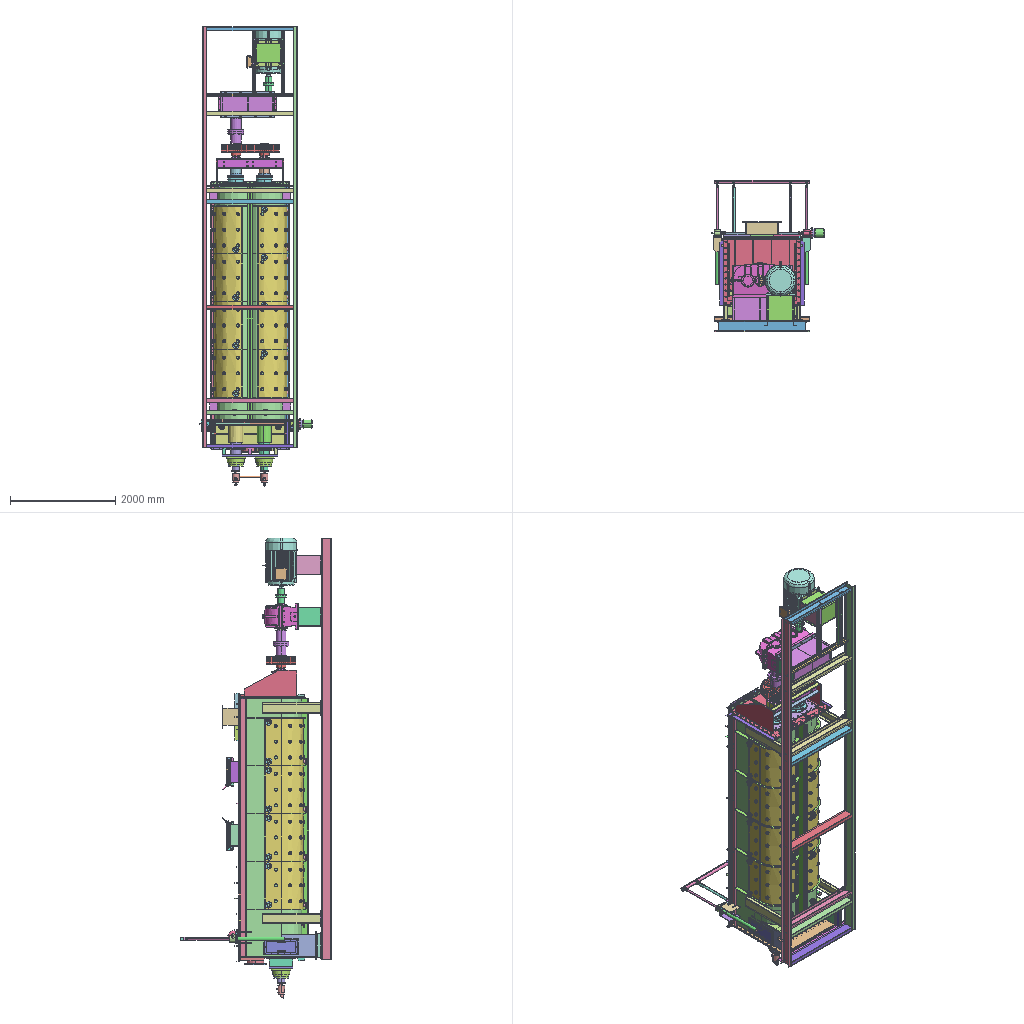Assembly | SolidWorks | 78 different items | 255 placed | box 2141 x 2886 x 8740 mm
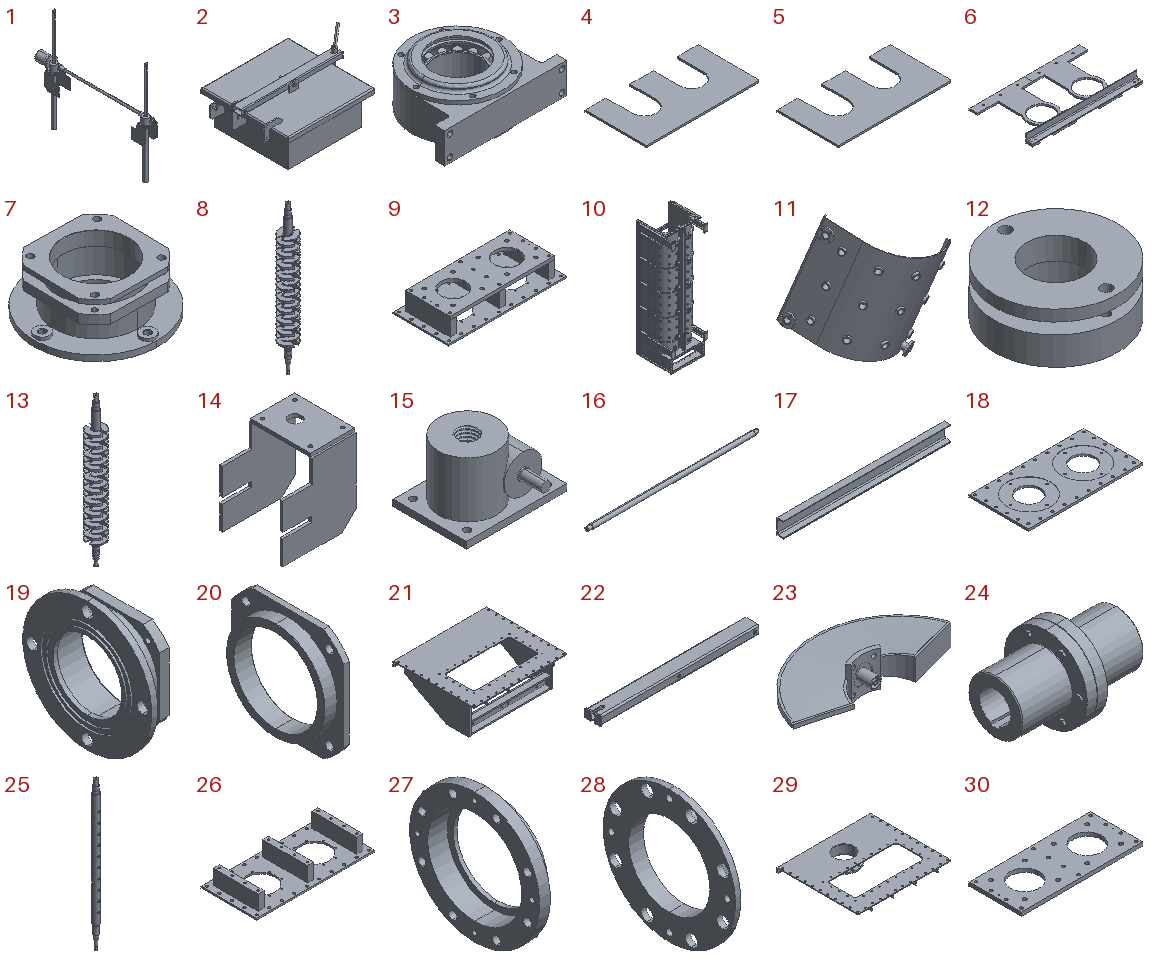Parts list (item | name | quantity | parent item | size | volume | features):
1 | (subassembly) | x1 | - | 241 x 2141 x 1901 mm | 19247413 mm3 | features AEMSimFeature 1
2 | (subassembly) | x2 | - | 610.405 x 476 x 304.855 mm | 2318365 mm3 | features AEMSimFeature 1, CompositeCurve 1
3 | (subassembly) | x2 | - | 480 x 370 x 194.8 mm | 12671030 mm3 | -
4 | (subassembly) | x1 | - | 1290 x 700 x 80 mm | 13949366 mm3 | features AEMSimFeature 1
5 | (subassembly) | x1 | in 4 | 1290 x 700 x 80 mm | 13949366 mm3 | features AEMSimFeature 1, MirrorCompFeat 1, ReferencePattern 1
6 | (subassembly) | x1 | - | 1300 x 750 x 100 mm | 9468918 mm3 | features HoleWzd 2, LPattern 2, AEMSimFeature 1
7 | (subassembly) | x2 | - | 420 x 420 x 162 mm | 4466169 mm3 | features ReferencePattern 3, AEMSimFeature 1, LocalCirPattern 1
8 | (subassembly) | x1 | - | - | 287612540 mm3 | features ReferencePattern 36, LocalLPattern 4, AEMSimFeature 1, RefAxis 1
9 | (subassembly) | x1 | - | 1185 x 560 x 198 mm | 31946209 mm3 | features AEMSimFeature 1
10 | (subassembly) | x1 | - | 1600 x 1565 x 4990 mm | 308843646 mm3 | features ReferencePattern 19, LocalLPattern 6, MirrorCompFeat 3, AEMSimFeature 1
11 | (subassembly) | x8 | in 10 | 940.727 x 808.112 x 1146 mm | 7168589 mm3 | features ReferencePattern 10, LocalLPattern 2, AEMSimFeature 1, LocalCirPattern 1, MirrorCompFeat 1
12 | (subassembly) | x2 | - | 110 x 110 x 45 mm | 226861 mm3 | features AEMSimFeature 1
13 | (subassembly) | x1 | - | - | 286429521 mm3 | features ReferencePattern 36, LocalLPattern 4, CompositeCurve 2, AEMSimFeature 1, RefAxis 1
14 | - | x1 | in 1 | 258 x 222 x 292 mm | 1584806 mm3 | features ICE 2, Chamfer 1, Cut 1, Extrusion 1, HoleWzd 1, MirrorSolid 1
15 | - | x1 | in 1 | - | 2041758 mm3 | features ICE 6, Extrusion 1, Helix 1, MirrorSolid 1, RefAxis 1, SweepCut 1
16 | - | x1 | in 1 | 1476 x 40 x 40 mm | 1810594 mm3 | features Chamfer 1, ICE 1, MirrorPattern 1, Revolution 1
17 | - | x3 | in 10 | 1300 x 53 x 120 mm | 1996260 mm3 | features WeldMemberFeat 1, WeldmentFeature 1
18 | - | x1 | - | 1140 x 590 x 22 mm | 12045594 mm3 | features ICE 3, CirPattern 2, HoleWzd 2, RefAxis 2, Extrusion 1
19 | - | x2 | in 7 | 116 x 420 x 420 mm | 3215271 mm3 | features ICE 4, Chamfer 2, CirPattern 2, HoleWzd 1, RefAxis 1, Revolution 1
20 | - | x2 | in 7 | 48 x 300 x 300 mm | 1152473 mm3 | features Chamfer 3, ICE 2, CirPattern 1, RefAxis 1, Revolution 1
21 | - | x1 | - | 1448 x 1250 x 512 mm | 47295525 mm3 | features ICE 13, LPattern 8, Chamfer 5, HoleWzd 4, MirrorPattern 3, MirrorSolid 2, Extrusion 1, Fillet 1
22 | - | x2 | in 2 | 554 x 54 x 30.061 mm | 237150 mm3 | features Cut 2, ICE 2, MirrorSolid 1, WeldMemberFeat 1, WeldmentFeature 1
23 | - | x80 | in 8, 13 | 715.716 x 337.387 x 160 mm | 3757176 mm3 | features ICE 17, MoveFace 13, DeleteBody 4, Chamfer 2, OffsetRefSurface 2, Split 2, Thicken 2, Blend 1, CirPattern 1, CombineBodies 1, Extrusion 1, MirrorSolid 1, Punch 1, RefAxis 1, RevCut 1, WeldmentFeature 1
24 | - | x1 | - | 294 x 200 x 200 mm | 3610457 mm3 | features ICE 15, Chamfer 6, Revolution 3, CirPattern 2, Fillet 2
25 | - | x1 | in 8 | 265 x 265 x 6370 mm | 136126152 mm3 | features ICE 15, LPattern 6, MirrorPattern 5, Fillet 2, HoleWzd 2, MoveFace 2, RefAxis 2, Chamfer 1, CombineBodies 1, Extrusion 1, MoveCopyBody 1, Revolution 1, Split 1, WeldBeadFeat 1, WeldmentFeature 1
26 | - | x1 | in 9 | 1185 x 560 x 166 mm | 20349216 mm3 | features ICE 3, HoleWzd 2, LPattern 2, CirPattern 1, Extrusion 1, MirrorPattern 1, RefAxis 1
27 | - | x2 | - | 65 x 365 x 365 mm | 1770977 mm3 | features CirPattern 1, HoleWzd 1, ICE 1, RefAxis 1, Revolution 1
28 | - | x3 | - | 41 x 365 x 365 mm | 1248338 mm3 | features ICE 2, Revolution 1
29 | - | x1 | - | 1448 x 1250 x 147 mm | 19462200 mm3 | features ICE 12, LPattern 7, Chamfer 4, MirrorPattern 2, MirrorSolid 2, Extrusion 1, Fillet 1, HoleWzd 1
30 | - | x1 | in 9 | 1050 x 450 x 32 mm | 11596993 mm3 | features ICE 3, MirrorPattern 3, CirPattern 1, Extrusion 1, HoleWzd 1
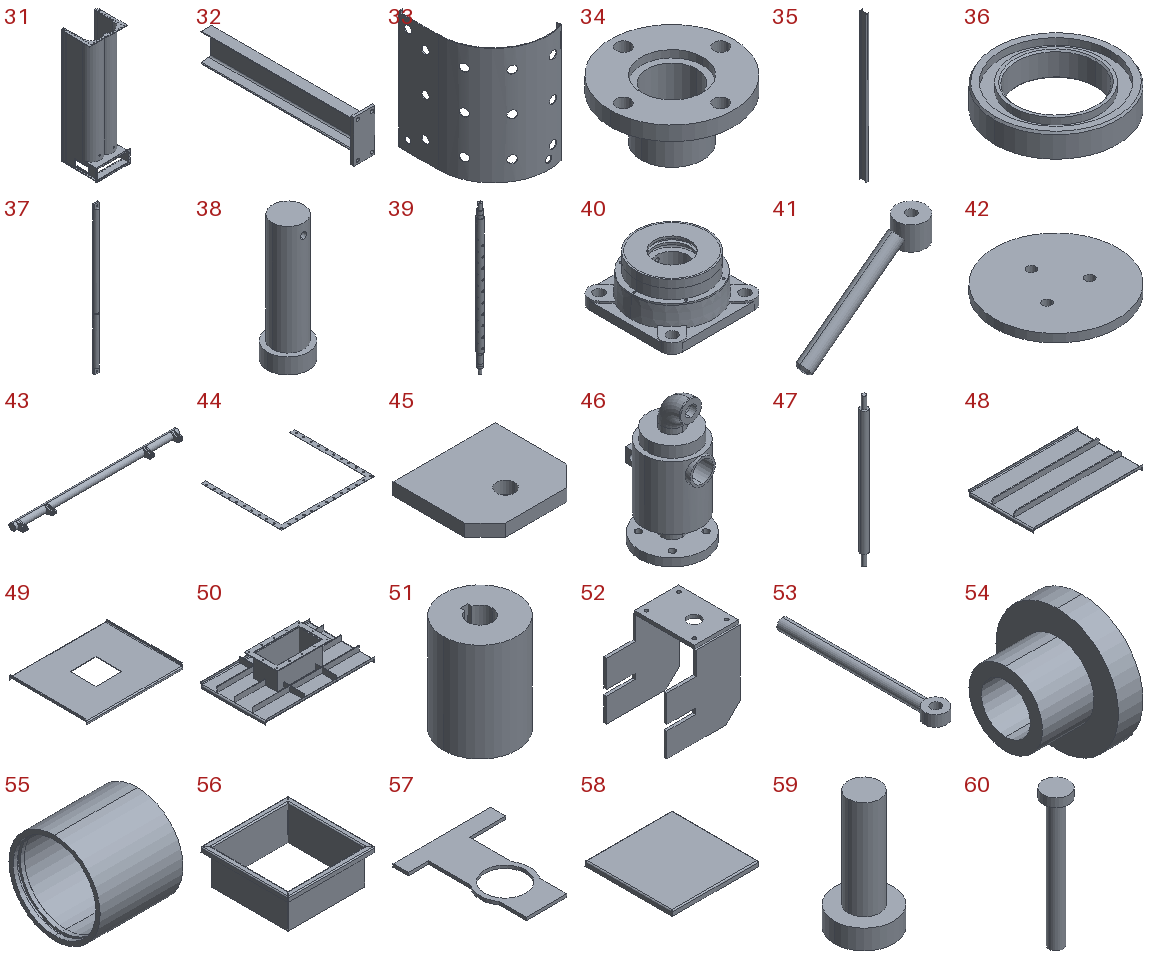31 | - | x1 | in 10 | 1600 x 1465 x 4987 mm | 200673004 mm3 | features ICE 14, HoleWzd 6, MirrorPattern 6, LPattern 5, CombineBodies 3, MirrorSolid 3, MoveFace 3, Extrusion 1, MoveCopyBody 1, Split 1
32 | - | x4 | in 10 | 150 x 1120 x 300 mm | 4040615 mm3 | features HoleWzd 1, ICE 1, MirrorPattern 1, WeldMemberFeat 1, WeldmentFeature 1
33 | - | x8 | in 11 | 548.116 x 742 x 900 mm | 6001500 mm3 | features EdgeFlange 2, ICE 2, RevCut 2, CirPattern 1, FlatPattern 1, LPattern 1, SMBaseFlange 1, SheetMetal 1
34 | - | x26 | in 10, 11 | 120 x 120 x 57 mm | 161025 mm3 | features ExtruThin 1, HoleWzd 1, ICE 1
35 | - | x1 | in 10 | 100 x 200 x 4480 mm | 12833917 mm3 | features Extrusion 1, MoveFace 1
36 | - | x3 | in 8, 13 | 85 x 85 x 17 mm | 42385 mm3 | features Chamfer 2, ICE 2, Extrusion 1
37 | - | x2 | - | 50 x 50 x 1600 mm | 3004412 mm3 | features HoleWzd 2, ICE 2, MirrorPattern 2, Extrusion 1
38 | - | x2 | - | 26 x 26 x 80 mm | 27050 mm3 | features ICE 2, Extrusion 1
39 | - | x1 | in 13 | 265 x 265 x 6190 mm | 134783572 mm3 | features ICE 16, HoleWzd 4, LPattern 4, MirrorPattern 4, Chamfer 2, CombineBodies 2, Fillet 2, MoveFace 2, RefAxis 2, CirPattern 1, DeleteBody 1, Extrusion 1, MoveCopyBody 1, Revolution 1, Split 1, WeldmentFeature 1
40 | - | x2 | - | 370 x 370 x 185 mm | 8271965 mm3 | features Revolution 5, RevCut 3, Boss 2, CirPattern 2, ICE 2, Cut 1, Extrusion 1, HoleWzd 1, RevolutionThin 1
41 | - | x2 | in 2 | 107.206 x 25 x 73.855 mm | 19838 mm3 | features Chamfer 1, Extrusion 1, HoleWzd 1, Revolution 1
42 | - | x1 | in 13 | 150 x 150 x 10 mm | 173864 mm3 | features BaseBody 1
43 | - | x1 | - | 1806 x 139 x 73 mm | 3217271 mm3 | features ICE 3, LPattern 2, MirrorSolid 2, HoleWzd 1, WeldMemberFeat 1, WeldmentFeature 1
44 | - | x2 | in 10 | 1448 x 1250 x 3 mm | 798363 mm3 | features Extrusion 1
45 | - | x2 | in 2 | 50 x 45 x 6 mm | 12518 mm3 | features Chamfer 1, Cut 1, Extrusion 1
46 | - | x2 | - | 150 x 170 x 315 mm | 2389466 mm3 | features ICE 8, CirPattern 1, Extrusion 1, HoleWzd 1, Sweep 1, SweepCut 1
47 | - | x1 | - | 30 x 30 x 615 mm | 384138 mm3 | features ICE 2, Extrusion 1
48 | - | x2 | - | 1492 x 898 x 110 mm | 11274482 mm3 | features Chamfer 2, EdgeFlange 2, BossThin 1, FlatPattern 1, SMBaseFlange 1, SheetMetal 1, WeldmentFeature 1
49 | - | x2 | - | 1492 x 1200 x 74 mm | 10683181 mm3 | features EdgeFlange 2, FlatPattern 1, ICE 1, SMBaseFlange 1, SheetMetal 1
50 | - | x1 | - | 1492 x 898 x 350 mm | 16578129 mm3 | features BossThin 2, EdgeFlange 2, HoleWzd 2, MirrorSolid 2, Cut 1, FlatPattern 1, ICE 1, LPattern 1, MirrorPattern 1, SMBaseFlange 1, SheetMetal 1
51 | - | x2 | in 1 | 60 x 60 x 80 mm | 183532 mm3 | features ICE 4, Extrusion 1
52 | - | x1 | in 1 | 258 x 222 x 292 mm | 1584806 mm3 | features ICE 2, Chamfer 1, Cut 1, Extrusion 1, HoleWzd 1, MirrorSolid 1
53 | - | x2 | in 2 | 20 x 150 x 10 mm | 12716 mm3 | features Extrusion 1, ICE 1, Revolution 1
54 | - | x8 | in 7 | 31 x 50 x 50 mm | 24606 mm3 | features Chamfer 1, Revolution 1
55 | - | x2 | in 8, 13 | 200 x 220 x 220 mm | 1255193 mm3 | features ICE 2, Revolution 1
56 | - | x2 | in 2 | 460 x 460 x 183 mm | 1117648 mm3 | features FlatPattern 4, ICE 1, SMBaseFlange 1, SMMiteredFlange 1, SheetMetal 1
57 | - | x2 | in 6 | 650 x 750 x 20 mm | 3819673 mm3 | features ICE 2, Extrusion 1
58 | - | x2 | in 2 | 476 x 476 x 28 mm | 807964 mm3 | features CornerFeat 4, FlatPattern 1, SMBaseFlange 1, SMMiteredFlange 1, SheetMetal 1
59 | - | x4 | in 2 | 15 x 15 x 30 mm | 2140 mm3 | features Extrusion 1, ICE 1
60 | - | x4 | in 2 | 15 x 15 x 80 mm | 4653 mm3 | features Extrusion 1, ICE 1
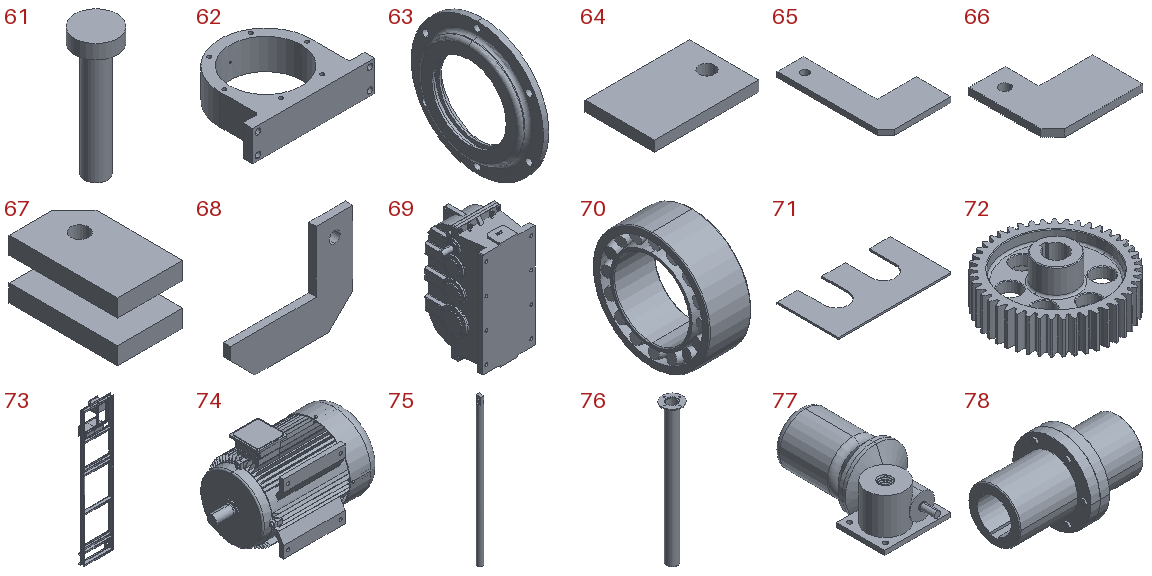61 | - | x2 | in 2 | 15 x 15 x 45 mm | 2894 mm3 | features Extrusion 1, ICE 1
62 | - | x2 | in 3 | 480 x 370 x 120 mm | 7370776 mm3 | features HoleWzd 3, ICE 2, CirPattern 1, Extrusion 1, Fillet 1, RefAxis 1
63 | - | x4 | in 3 | 47.4 x 360 x 360 mm | 1531898 mm3 | features ICE 1, Revolution 1
64 | - | x2 | in 2 | 60 x 40 x 6 mm | 14018 mm3 | features Extrusion 1, ICE 1
65 | - | x2 | in 2 | 75 x 125 x 6 mm | 32618 mm3 | features Chamfer 1, Extrusion 1, ICE 1
66 | - | x2 | in 2 | 75 x 70 x 6 mm | 23195 mm3 | features Chamfer 1, Extrusion 1, ICE 1
67 | - | x2 | in 5 | 60 x 100 x 54 mm | 178758 mm3 | features Chamfer 1, Extrusion 1, ICE 1, MirrorSolid 1
68 | - | x2 | in 2 | 100 x 6 x 80 mm | 24218 mm3 | features Chamfer 2, Extrusion 1, ICE 1
69 | - | x1 | - | 780 x 662 x 1105 mm | 238167448 mm3 | features ICE 43, Extrusion 14, Fillet 9, CirPattern 5, Chamfer 4, MirrorPattern 4, DeleteBody 2, LPattern 1, RefAxis 1, Revolution 1
70 | - | x2 | in 3 | 100 x 280 x 280 mm | 2236455 mm3 | features Revolution 4, Fillet 2, CirPattern 1, MirrorPattern 1, MirrorSolid 1
71 | - | x1 | in 5 | 1290 x 700 x 20 mm | 13591851 mm3 | features Extrusion 1, Fillet 1, ICE 1
72 | - | x2 | - | 563.903 x 563.597 x 220 mm | 18785882 mm3 | features ICE 8, Chamfer 2, CirPattern 1, Extrusion 1, Fillet 1, RefAxis 1
73 | - | x1 | - | 1791 x 685 x 8000 mm | 140497975 mm3 | features MoveFace 19, MoveCopyBody 18, ICE 10, MirrorSolid 9, WeldMemberFeat 7, 3DProfileFeature 3, Cut 3, DeleteBody 2, Shell 2, Punch 1, WeldmentFeature 1
74 | - | x1 | - | 1055 x 665 x 715 mm | 197436858 mm3 | features Boss 17, Cut 5, Revolution 5, Fillet 4, Chamfer 3, CirPattern 3, RevCut 2, 3DProfileFeature 1, LPattern 1, MirrorPattern 1, MoveCopyBody 1
75 | - | x2 | in 1 | 40 x 40 x 1100 mm | 1353457 mm3 | features ICE 2, Extrusion 1
76 | - | x2 | in 1 | 130 x 130 x 909 mm | 633307 mm3 | features ICE 2, ExtruThin 1, HoleWzd 1
77 | - | x1 | in 1 | 236 x 443.1 x 200 mm | 7884853 mm3 | features ICE 9, Blend 2, Fillet 2, Extrusion 1, Helix 1, RefAxis 1, SweepCut 1
78 | - | x1 | - | 474 x 300 x 300 mm | 12928515 mm3 | features ICE 15, Chamfer 6, Revolution 3, CirPattern 2, Fillet 2
Mates (type | each side: item.copy, entity, surface, feature):
In the top assembly
Coincident | 44.1 face plane Boss-Extrude1 | 21.1 face plane Boss-Extrude1
Concentric | 31.1 face cylinder M22 Tapped Hole3 | 21.1 face cylinder Cut-Extrude2
Concentric | 31.1 face cylinder Mirror4 | 21.1 face cylinder Cut-Extrude2
Coincident | 44.2 face plane Boss-Extrude1 | 29.1 face plane Boss-Extrude1
Concentric | 31.1 face cylinder M22 Tapped Hole1 | 29.1 face cylinder Cut-Extrude2
Concentric | 31.1 face cylinder LPattern1 | 29.1 face cylinder Cut-Extrude2
Coincident | 27.1 face plane Revolve1 | 28.1 face plane Revolve1
Concentric | 27.1 face cylinder Revolve1 | 28.1 face cylinder Revolve1
DistanceDim | 27.2 face plane Revolve1 | 28.2 face plane Revolve1
Concentric | 27.2 face cylinder Revolve1 | 28.2 face cylinder Revolve1
DistanceDim | assembly face | assembly face
Concentric | assembly face | assembly face
DistanceDim | 28.3 face plane Revolve1 | 27.1 face plane Revolve1
Concentric | 27.1 face cylinder Revolve1 | 28.3 face cylinder Revolve1
DistanceDim | 25.1 face plane Boss-Extrude7 | 18.1 face plane Boss-Extrude1
DistanceDim | 39.1 face plane Boss-Extrude7 | 18.1 face plane Boss-Extrude1
Concentric | 39.1 face cylinder Boss-Extrude4 | 70.1 face cylinder Revolve1
Coincident | 39.1 face plane Boss-Extrude5 | 70.1 face plane Revolve1
Concentric | 25.1 face cylinder Boss-Extrude1 | 70.2 face cylinder Revolve1
Coincident | 25.1 face plane Boss-Extrude5 | 70.2 face plane Revolve1
DistanceDim | 26.1 face plane Boss-Extrude1 | 29.1 face plane Boss-Extrude1
Concentric | 29.1 face cylinder M20 Tapped Hole1 | 26.1 face cylinder Cut-Extrude1
Concentric | 29.1 face cylinder LPattern12 | 26.1 face cylinder Cut-Extrude1
DistanceDim | 27.2 face plane Revolve1 | 26.1 face plane Boss-Extrude1
Concentric | 26.1 face cylinder Cut-Extrude2 | 27.2 face cylinder Revolve1
Concentric | 26.1 face cylinder Mirror1 | 27.2 face cylinder Cut-Extrude1
DistanceDim | 27.1 face plane Revolve1 | 26.1 face plane Boss-Extrude1
Concentric | 26.1 face cylinder Cut-Extrude2 | 27.1 face cylinder Revolve1
Concentric | 30.1 face cylinder Mirror3 | 40.1 face cylinder Base-Extrude
Concentric | 30.1 face cylinder Mirror1 | 40.1 face cylinder Base-Extrude
Coincident | 30.1 face plane Boss-Extrude1 | 40.1 face plane Base-Extrude
Concentric | 30.1 face cylinder M36 Tapped Hole1 | 40.2 face cylinder Base-Extrude
Concentric | 30.1 face cylinder CirPattern1 | 40.2 face cylinder Base-Extrude
Coincident | 30.1 face plane Boss-Extrude1 | 40.2 face plane Base-Extrude
Concentric | 25.1 face cylinder Revolve2 | 46.1 face cylinder Cut-Extrude2
Parallel | 30.1 face plane Boss-Extrude1 | 46.1 face plane Boss-Extrude4
Coincident | 25.1 face plane Revolve2 | 46.1 face plane Boss-Extrude1
Concentric | 39.1 face cylinder Revolve1 | 46.2 face cylinder Sweep1
Parallel | 30.1 face plane Boss-Extrude1 | 46.2 face plane Boss-Extrude4
Coincident | 39.1 face plane Revolve1 | 46.2 face plane Boss-Extrude1
Concentric | 46.2 face cylinder Cut-Extrude5 | 47.1 face cylinder Boss-Extrude1
Coincident | 46.2 face plane Boss-Extrude4 | 47.1 face plane Boss-Extrude1
Parallel | 31.1 face plane Boss-Extrude6 | 57.1 face plane
Coincident | 31.1 face plane Boss-Extrude3 | 57.1 face plane
DistanceDim | 31.1 face plane Mirror2 | 48.1 face plane Base-Flange1
Coincident | 17.1 edge | 48.1 face plane Edge-Flange2
Width | 48.1 face plane Edge-Flange3 | 48.1 face plane Edge-Flange3 | 31.1 face plane Boss-Extrude1 | 31.1 face plane Boss-Extrude1
Coincident | 48.1 face plane Edge-Flange3 | 49.1 face plane Edge-Flange3
Coincident | 48.1 face plane Edge-Flange2 | 49.1 face plane Edge-Flange2
Coincident | 48.1 face plane Base-Flange1 | 49.1 face plane Base-Flange1
Coincident | 49.2 face plane Base-Flange1 | 50.1 face plane Base-Flange1
Coincident | 49.2 face plane Edge-Flange3 | 50.1 face plane Edge-Flange3
Coincident | 49.2 face plane Edge-Flange2 | 50.1 face plane Edge-Flange2
Concentric | 37.1 face cylinder | 38.1 face cylinder Boss-Extrude1
Parallel | 37.2 face plane | 37.1 face plane
Width | 31.1 face plane Boss-Extrude4 | 31.1 face plane Mirror1 | 71.1 face plane Boss-Extrude1 | 71.1 face plane Boss-Extrude1
DistanceDim | 31.1 face plane Boss-Extrude3 | 71.1 face plane Boss-Extrude1
LimitDistanceDim | 71.1 face plane Boss-Extrude1 | 31.1 face plane Boss-Extrude6
Width | 37.2 face plane | 37.2 face plane | 67.1 face plane Boss-Extrude1 | 67.1 face plane Mirror1
Concentric | 67.1 face cylinder Mirror1 | 37.2 face cylinder
Parallel | 67.1 face plane Mirror1 | 37.2 face plane
Concentric | 67.1 face cylinder Mirror1 | 38.2 face cylinder Boss-Extrude1
Coincident | 67.1 face plane Mirror1 | 38.2 face plane Boss-Extrude2
Concentric | 67.2 face cylinder Cut-Extrude1 | 37.1 face cylinder
Width | 67.2 face plane Mirror1 | 67.2 face plane Boss-Extrude1 | 37.1 face plane | 37.1 face plane
Coincident | 67.2 face plane Boss-Extrude1 | 38.1 face plane Boss-Extrude2
Concentric | 37.2 face cylinder | 43.1 face cylinder Ø16.5 (16.5) Diameter Hole1
Width | 43.1 face plane Boss-Extrude1 | 43.1 face plane LPattern1 | 37.2 face plane | 37.2 face plane
Parallel | 37.2 face plane | 43.1 edge
Parallel | 37.2 face plane | 43.1 plane
Parallel | 31.1 face plane Mirror2 | 77.1 face plane Boss-Extrude1
Width | 77.1 face plane Boss-Extrude1 | 15.1 face plane Boss-Extrude1 | 31.1 face plane Boss-Extrude8 | 31.1 face plane Mirror2
Concentric | 43.1 face cylinder LPattern2 | 75.1 face cylinder Cut-Extrude2
DistanceDim | 77.1 face plane Boss-Extrude1 | 31.1 face plane Mirror2
Coincident | 49.2 face plane Base-Flange1 | 56.1 face plane Cut-Extrude1
Coincident | 49.2 face plane Cut-Extrude1 | 56.1 face plane Miter Flange1 | 2 times
Coincident | 49.1 face plane Cut-Extrude1 | 56.2 face plane Miter Flange1 | 2 times
Coincident | 49.1 face plane Base-Flange1 | 56.2 face plane Cut-Extrude1
Coincident | 21.1 face plane Boss-Extrude1 | 18.1 face plane Boss-Extrude1
Concentric | 18.1 face cylinder Cut-Extrude2 | 25.1 face cylinder Boss-Extrude6
Concentric | assembly face | 25.1 face cylinder Boss-Extrude5
Coincident | 18.1 face plane Cut-Extrude3 | 19.1 face plane Revolve1
Concentric | 18.1 face cylinder Cut-Extrude2 | 19.1 face cylinder Revolve1
Concentric | 19.1 face cylinder Revolve1 | 55.1 face cylinder Revolve1
Concentric | 31.1 face cylinder Boss-Extrude1 | 19.1 face cylinder Revolve1
Concentric | 19.1 face cylinder CirPattern1 | 18.1 face cylinder CirPattern1
Concentric | 55.2 face cylinder Revolve1 | 19.2 face cylinder Revolve1
Coincident | 18.1 face plane Cut-Extrude3 | 19.2 face plane Revolve1
Concentric | 18.1 face cylinder CircPattern2 | 19.2 face cylinder CirPattern1
Parallel | 21.1 face plane Boss-Extrude7 | 62.1 face plane Boss-Extrude1
Parallel | 21.1 face plane Boss-Extrude7 | 62.2 face plane Boss-Extrude1
Concentric | 31.1 face cylinder Boss-Extrude1 | 25.1 face cylinder Boss-Extrude7
Coincident | 48.1 face plane Base-Flange1 | 48.2 face plane
Coincident | 48.1 face plane Edge-Flange3 | 48.2 face plane
Coincident | 48.1 face plane Edge-Flange2 | 48.2 face plane
Concentric | 25.1 face cylinder Boss-Extrude1 | 72.1 face cylinder Cut-Extrude4
Concentric | 39.1 face cylinder Boss-Extrude1 | 72.2 face cylinder Boss-Extrude2
Coincident | 72.1 face plane Boss-Extrude1 | 72.2 face plane Boss-Extrude1
GearDim | 72.1 face cylinder Boss-Extrude2 | 72.2 face cylinder Boss-Extrude2
Coincident | 25.1 face plane Cut-Extrude6 | 72.1 face plane Cut-Extrude6
Coincident | 39.1 face plane Cut-Extrude6 | 72.2 face plane Cut-Extrude6
Concentric | 25.1 face cylinder Boss-Extrude1 | 69.1 face cylinder Boss-Extrude79
Parallel | 21.1 face plane Boss-Extrude7 | 69.1 face plane Boss-Extrude1
Concentric | 69.1 face cylinder Boss-Extrude76 | 74.1 face cylinder Revolve1
Parallel | 69.1 face plane Boss-Extrude1 | 74.1 face plane Extrude2
Concentric | 69.1 face cylinder Boss-Extrude79 | 78.1 face cylinder Cut-Extrude5
Coincident | 69.1 face plane Boss-Extrude80 | 78.1 face plane Cut-Extrude7
DistanceDim | 78.1 face plane Revolve1 | 69.1 face plane Boss-Extrude78
DistanceDim | 72.1 face plane Boss-Extrude2 | 78.1 face plane Revolve2
Concentric | 74.1 face cylinder Revolve1 | 24.1 face cylinder Cut-Extrude5
Coincident | 74.1 face plane Cut-Extrude1 | 24.1 face plane Cut-Extrude7
DistanceDim | 74.1 face plane Revolve1 | 24.1 face plane Revolve1
DistanceDim | 69.1 face plane Mirror6 | 24.1 face plane Revolve2
In subassembly 2
Coincident | 56.3 face plane Miter Flange1 | 58.1 face plane Base-Flange1
Width | 58.1 face plane Miter Flange1 | 58.1 face plane Miter Flange1 | 56.3 face plane Miter Flange1 | 56.3 face plane Miter Flange1
Coincident | 58.1 face plane Base-Flange1 | 68.1 face plane Boss-Extrude1
DistanceDim | 58.1 face plane Miter Flange1 | 68.1 face plane Boss-Extrude1
Parallel | 58.1 face plane Base-Flange1 | 22.1 face plane Structural Member2
Width | 58.1 face plane Miter Flange1 | 58.1 face plane Miter Flange1 | 22.1 face plane Structural Member2 | 22.1 face plane Structural Member2
Coincident | 68.1 face plane Boss-Extrude1 | 59.1 face plane Boss-Extrude2
Concentric | 66.1 face cylinder Cut-Extrude1 | 59.2 face cylinder Boss-Extrude1
Coincident | 66.1 face plane Boss-Extrude1 | 59.2 face plane Boss-Extrude2
Coincident | 68.1 face plane Boss-Extrude1 | 22.1 face plane Structural Member2
Width | 22.1 face plane Structural Member2 | 22.1 face plane Structural Member2 | 58.1 face plane Miter Flange1 | 58.1 face plane Miter Flange1
Coincident | 22.1 face plane Structural Member2 | 65.1 face plane Boss-Extrude1
Concentric | 22.1 face cylinder Cut-Extrude2 | 65.1 face cylinder Cut-Extrude1
DistanceDim | 22.1 face plane Structural Member2 | 58.1 face plane Base-Flange1
Concentric | 65.1 edge | 60.1 face cylinder Boss-Extrude1
DistanceDim | 45.1 face plane Boss-Extrude1 | 22.1 face plane Structural Member2
Coincident | 58.1 face plane Base-Flange1 | 45.1 face plane Boss-Extrude1
Width | 58.1 face plane Miter Flange1 | 58.1 face plane Miter Flange1 | 45.1 face plane Boss-Extrude1 | 45.1 face plane Boss-Extrude1
Coincident | 56.3 face plane Miter Flange1 | 64.1 face plane Boss-Extrude1
DistanceDim | 64.1 face plane Boss-Extrude1 | 56.3 face plane Miter Flange1
DistanceDim | 58.1 face plane Base-Flange1 | 64.1 face plane Boss-Extrude1
Concentric | 45.1 face cylinder Cut-Extrude1 | 60.2 face cylinder Boss-Extrude1
Coincident | 45.1 face plane Boss-Extrude1 | 60.2 face plane Boss-Extrude2
Concentric | 64.1 face cylinder Cut-Extrude1 | 61.1 face cylinder Boss-Extrude1
Coincident | 64.1 face plane Boss-Extrude1 | 61.1 face plane Boss-Extrude2
Concentric | 61.1 face cylinder Boss-Extrude1 | 53.1 face cylinder Cut-Extrude1
Concentric | 53.1 face cylinder Revolve1 | 41.1 face cylinder M10 Tapped Hole1
Coincident | 22.1 face plane Structural Member2 | 41.1 face plane Boss-Extrude1
In subassembly 3
Concentric | 62.3 face cylinder Boss-Extrude1 | 70.3 face cylinder Revolve1
DistanceDim | 62.3 face plane Boss-Extrude1 | 70.3 face plane Revolve3
Concentric | 70.3 face cylinder Revolve1 | 63.1 face cylinder Revolve1
Coincident | 62.3 face plane Boss-Extrude1 | 63.1 face plane Revolve1
Concentric | 62.3 face cylinder Boss-Extrude1 | 63.2 face cylinder Revolve1
Coincident | 62.3 face plane Boss-Extrude1 | 63.2 face plane Revolve1
In subassembly 6
Coincident | 57.2 face plane | 57.3 face plane | 3 times
In subassembly 1
Concentric | 77.2 face cylinder Boss-Extrude7 | 16.1 face cylinder Revolve1
Concentric | 16.1 face cylinder Revolve1 | 51.1 face cylinder Cut-Extrude2 | 2 times
Coincident | 16.1 face plane Revolve1 | 51.1 face plane Boss-Extrude1
DistanceDim | 77.2 face plane Boss-Extrude7 | 16.1 face plane Revolve1
Concentric | 16.1 face cylinder Revolve1 | 51.2 face cylinder Cut-Extrude2
Coincident | 16.1 face plane Revolve1 | 51.2 face plane Boss-Extrude1
DistanceDim | 15.2 face plane Mirror3 | 16.1 face plane Revolve1
Concentric | 51.2 face cylinder Cut-Extrude1 | 15.2 face cylinder Mirror3
Concentric | 15.2 face cylinder Cut-Extrude2 | 75.2 face cylinder Boss-Extrude1
Concentric | 77.2 face cylinder Cut-Extrude2 | 75.3 face cylinder Boss-Extrude1 | 2 times
Coincident | 77.2 face plane Boss-Extrude1 | 15.2 face plane Boss-Extrude1
Coincident | 15.2 face plane Boss-Extrude1 | 52.1 face plane Boss-Extrude1 | 2 times
Concentric | 15.2 face cylinder Cut-Extrude1 | 52.1 face cylinder Ø12.0 (12) Diameter Hole1
Coincident | 77.2 face plane Boss-Extrude1 | 1.1 face
Parallel | 77.2 face plane Boss-Extrude1 | 1.1 face
Concentric | 77.2 face cylinder Cut-Extrude1 | 1.1 face
Concentric | 75.2 face cylinder Boss-Extrude1 | 76.1 face cylinder Thin Extrude1
Coincident | 52.1 face plane Boss-Extrude1 | 76.1 face plane Boss-Extrude2
Concentric | 75.3 face cylinder Boss-Extrude1 | 76.2 face cylinder Thin Extrude1
Coincident | 1.1 face | 76.2 face plane Boss-Extrude2
Coincident | 77.2 face plane Boss-Extrude1 | 14.1 face plane Boss-Extrude1
Parallel | 77.2 face plane Boss-Extrude1 | 14.1 face plane Boss-Extrude1
Concentric | 77.2 face cylinder Cut-Extrude1 | 14.1 face cylinder Ø12.0 (12) Hole1
In subassembly 8
Coincident | 25.2 face plane Cut-Extrude2 | 36.1 face plane Boss-Extrude1
Concentric | 25.2 face cylinder Cut-Extrude2 | 36.1 face cylinder Boss-Extrude1
Coincident | 25.2 face plane Cut-Extrude4 | 36.2 face plane Boss-Extrude1
Concentric | 25.2 face cylinder Cut-Extrude4 | 36.2 face cylinder Boss-Extrude1
Concentric | 25.2 face cylinder Cut-Extrude3 | 23.1 face cylinder Boss-Extrude6
Concentric | 25.2 face cylinder Boss-Extrude7 | 23.1 face cylinder Boss-Extrude1
Concentric | 25.2 face cylinder Cut-Extrude5 | 23.2 face cylinder Boss-Extrude6
Concentric | 25.2 face cylinder Boss-Extrude7 | 23.2 face cylinder Boss-Extrude1
Concentric | 25.2 face cylinder Mirror3 | 23.3 face cylinder Boss-Extrude6
Concentric | 25.2 face cylinder Boss-Extrude7 | 23.3 face cylinder Boss-Extrude1
Concentric | 25.2 face cylinder Boss-Extrude5 | 55.3 face cylinder Revolve1
Coincident | 25.2 face plane Boss-Extrude13 | 55.3 face plane Revolve1
Concentric | 25.2 face cylinder Mirror2 | 23.4 face cylinder Boss-Extrude6
Concentric | 25.2 face cylinder Boss-Extrude7 | 23.4 face cylinder Boss-Extrude1
In subassembly 10
Coincident | 35.1 face plane Boss-Extrude1 | 10.1 plane
Coincident | 31.2 face plane Boss-Extrude2 | 35.1 face plane Boss-Extrude1
DistanceDim | 35.1 face plane Boss-Extrude1 | 10.1 plane
Coincident | 31.2 face plane Boss-Extrude5 | 44.3 face plane Boss-Extrude1
Concentric | 31.2 face cylinder M22 Tapped Hole1 | 44.3 face cylinder Boss-Extrude1
Coincident | 31.2 face plane Boss-Extrude2 | 44.4 face plane Boss-Extrude1
Concentric | 44.4 face cylinder Boss-Extrude1 | 31.2 face cylinder Mirror4
Concentric | 31.2 face cylinder Boss-Extrude1 | 33.1 face cylinder Base-Bend1
Parallel | 31.2 face plane Boss-Extrude1 | 33.1 face plane Base-Flange1
Concentric | 31.2 face cylinder Boss-Extrude1 | 33.2 face cylinder Base-Bend1
Parallel | 31.2 face plane Boss-Extrude1 | 33.2 face plane Base-Flange1
Coincident | 31.2 face plane Boss-Extrude1 | 32.1 face plane Structural Member1
DistanceDim | 32.1 face plane Structural Member1 | 31.2 face plane Boss-Extrude3
DistanceDim | 32.1 face plane Boss-Extrude1 | 31.2 face plane Boss-Extrude6
Coincident | 31.2 face plane Mirror2 | 17.2 face plane Structural Member1
Coincident | 31.2 face plane Boss-Extrude1 | 17.2 face plane Structural Member1
DistanceDim | 31.2 face plane Boss-Extrude2 | 17.2 face plane Structural Member1
Concentric | 31.2 face cylinder Cut-Extrude12 | 34.1 face cylinder Extrude-Thin1
Coincident | 31.2 select_type:25 | 34.1 select_type:25
In subassembly 11
Concentric | 33.3 face cylinder Cut-Extrude2 | 34.1 face cylinder Extrude-Thin1
Coincident | 33.3 face plane Base-Flange1 | 34.1 face plane Extrude-Thin1
Concentric | 33.3 face cylinder Cut-Extrude2 | 34.2 face cylinder Extrude-Thin1
Coincident | 33.3 face plane Base-Flange1 | 34.2 face plane Extrude-Thin1
Concentric | 33.3 face cylinder Cut-Revolve2 | 34.3 face cylinder Extrude-Thin1
Tangent | 33.3 face cylinder Base-Bend1 | 34.3 face plane Extrude-Thin1
In subassembly 9
Coincident | 26.2 face plane Boss-Extrude2 | 30.2 face plane Boss-Extrude1
Width | 30.2 face plane Boss-Extrude1 | 30.2 face plane Boss-Extrude1 | 26.2 face plane Boss-Extrude2 | 26.2 face plane LPattern2
In subassembly 7
DistanceDim | 20.1 face plane Revolve1 | 19.3 face plane Revolve1
Concentric | 19.3 face cylinder Revolve1 | 20.1 face cylinder Revolve1
Concentric | 54.1 face cylinder Revolve1 | 19.3 face cylinder Cut-Extrude3
Coincident | 54.1 face plane Revolve1 | 19.3 face plane Revolve1
In subassembly 13
Coincident | 39.2 face plane Cut-Extrude9 | 36.2 face plane Boss-Extrude1
Concentric | 39.2 face cylinder Cut-Extrude9 | 36.2 face cylinder Boss-Extrude1
Concentric | 39.2 face cylinder Boss-Extrude7 | 13.1 face
Concentric | 36.2 face cylinder Boss-Extrude1 | 23.5 face cylinder Boss-Extrude6
Concentric | 39.2 face cylinder Boss-Extrude7 | 23.5 face cylinder Boss-Extrude1
Concentric | 39.2 face cylinder Mirror2 | 23.6 face cylinder Boss-Extrude6
Concentric | 39.2 face cylinder Boss-Extrude7 | 23.6 face cylinder Boss-Extrude1
Concentric | 39.2 face cylinder Boss-Extrude5 | 55.4 face cylinder Revolve1
Coincident | 39.2 face plane Boss-Extrude13 | 55.4 face plane Revolve1
Concentric | 39.2 face cylinder Mirror3 | 23.7 face cylinder Boss-Extrude6
Coincident | 39.2 face cylinder Boss-Extrude7 | 23.7 edge
Concentric | 39.2 face cylinder Cut-Extrude14 | 23.8 face cylinder Boss-Extrude6
Coincident | 39.2 face cylinder Boss-Extrude7 | 23.8 edge
Concentric | 39.2 face cylinder Boss-Extrude1 | 42.1 face cylinder Input1
Concentric | 39.2 face cylinder M10 Tapped Hole1 | 42.1 face cylinder Input1
In subassembly 5
Coincident | 71.2 face plane Boss-Extrude1 | 67.3 face plane Boss-Extrude1
DistanceDim | 71.2 edge | 67.3 face plane Boss-Extrude1
DistanceDim | 67.3 face plane Boss-Extrude1 | 71.2 face plane Boss-Extrude1